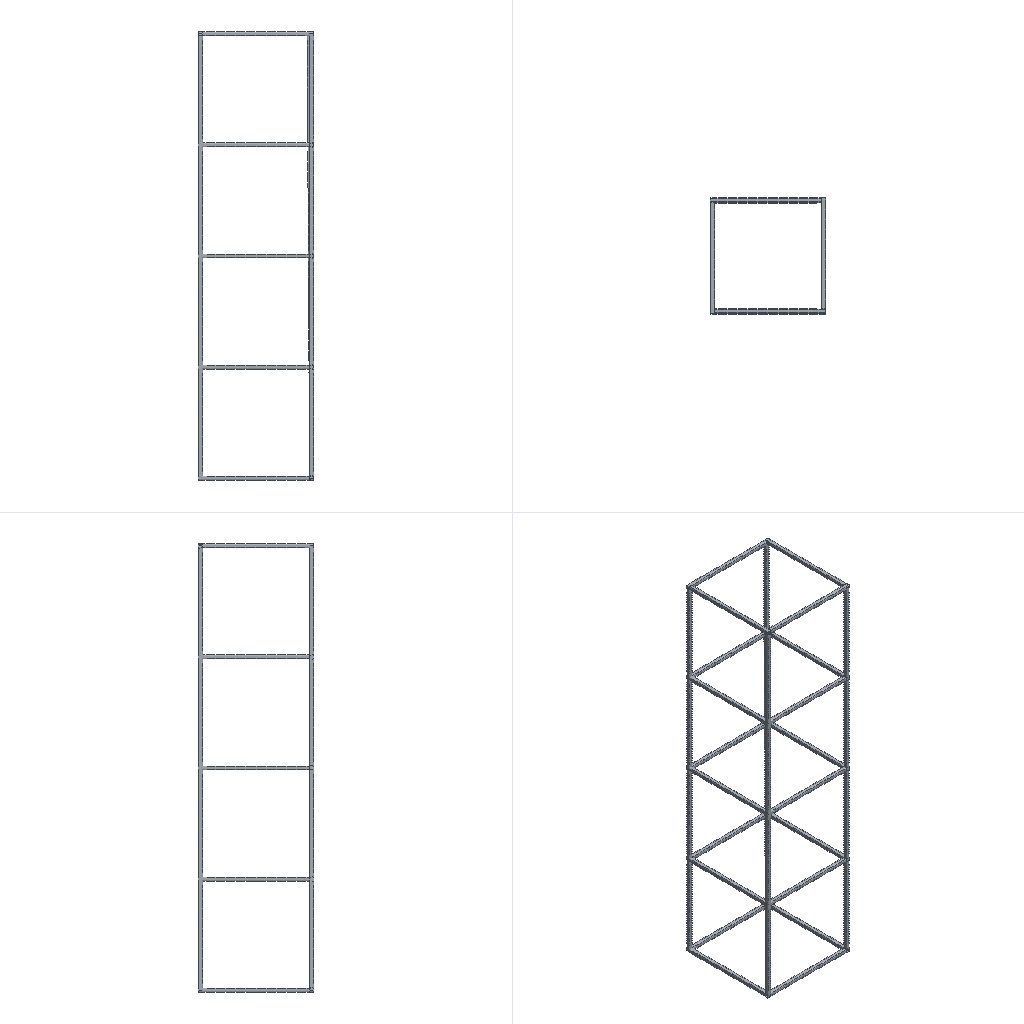Simulation study | ansys workbench
Ansys APDL input file, long lists of numbers shortened:
/batch
/config,noeldb,1     ! force off writing results to database
*get,_wallstrt,active,,time,wall
! ANSYS input file written by Workbench version 2022 R1
! File used for geometry attach:
/title,wbnew--____ (A5)
! ****** Begin Custom Load Command Snippet ******
/COM, ACT Extensions:
/COM,     LSDYNA, 2021.1
/COM,
! ****** End   Custom Load Command Snippet ******
*DIM,_wb_ProjectScratch_dir,string,248
_wb_ProjectScratch_dir(1) = ''
*DIM,_wb_SolverFiles_dir,string,248
_wb_SolverFiles_dir(1) = ''
*DIM,_wb_userfiles_dir,string,248
_wb_userfiles_dir(1) = ''
/com,--- Data in consistent NMM units. See Solving Units in the help system for more information.
/units,MPA
/nopr
/wb,file,start              !  signify a WB generated input file
/prep7
! Turn off shape checking because checks already performed inside WB mesher.
! See help system for more information.
SHPP,OFF,,NOWARN
/nolist
etcon,set             ! allow ANSYS to choose best KEYOP's for 180x elements, resets any applicable keyopt to MAPDL defaults
/com,*********** Nodes for the whole assembly ***********
nblock,3,,335992
(1i9,3e20.9e3)
        1     2.400000000E+02     2.588284271E+02     8.828427125E+00
! (305447 more lines like these left out)
-1
/wb,elem,start            !  set before creation of elements
/com,*********** Elements for Body 1 "__-FreeParts|__ 20 X 20 X 2.0(1)[4]" ***********
et,1,186
keyo,1,2,1          ! set full integration on SOLID186
eblock,19,solid,,1200
(19i9)
        1        1        1        1        0        0        0        0       20        0     9601    68809    69006    69556    69609    68858    68861    69555    69610
! (2399 more lines like these left out)
-1
/com,*********** Elements for Body 2 "__-FreeParts|__ 20 X 20 X 2.0(1)[2]" ***********
et,2,186
keyo,2,2,1          ! set full integration on SOLID186
eblock,19,solid,,1200
(19i9)
        2        2        2        2        0        0        0        0       20        0    13201    94369    94566    95116    95169    94418    94421    95115    95170
! (2399 more lines like these left out)
-1
/com,*********** Elements for Body 3 "__-FreeParts|__(__)1[9]" ***********
et,3,186
keyo,3,2,1          ! set full integration on SOLID186
eblock,19,solid,,1200
(19i9)
        3        3        3        3        0        0        0        0       20        0     6001    43099    44893    44700    43298    43246    44896    44699    43297
! (2399 more lines like these left out)
-1
/com,*********** Elements for Body 4 "__-FreeParts|__ 20 X 20 X 2.0(2)[4]" ***********
et,4,186
keyo,4,2,1          ! set full integration on SOLID186
eblock,19,solid,,1200
(19i9)
        4        4        4        4        0        0        0        0       20        0     3601    26359    27411    27360    26558    26506    27556    27359    26557
! (2399 more lines like these left out)
-1
/com,*********** Elements for Body 5 "__-FreeParts|__ 20 X 20 X 2.0(2)[2]" ***********
et,5,186
keyo,5,2,1          ! set full integration on SOLID186
eblock,19,solid,,1200
(19i9)
        5        5        5        5        0        0        0        0       20        0    15601   110860   112159   112156   111106   110958   112160   112153   111105
! (2399 more lines like these left out)
-1
! (19 more sections like these left out)
/wb,elem,end               !  done creating elements
/com,*********** Send User Defined Coordinate System(s) ***********
csys,0
toffst,273.15,  ! Temperature offset from absolute zero
/com,*********** Set Reference Temperature ***********
tref,22.
/wb,mat,start              !  starting to send materials
/com,*********** Send Materials ***********
Temperature = 'TEMP' ! Temperature
MP,DENS,1,7.85e-09,	! tonne mm^-3
MP,ALPX,1,1.2e-05,	! C^-1
MP,C,1,434000000,	! mm^2 s^-2 C^-1
MP,KXX,1,60.5,	! tonne mm s^-3 C^-1
MP,RSVX,1,0.00017,	! ohm mm
MP,EX,1,200000,	! tonne s^-2 mm^-1
MP,NUXY,1,0.3,
MP,MURX,1,10000,
Temperature = 'TEMP' ! Temperature
MP,DENS,2,7.85e-09,	! tonne mm^-3
MP,ALPX,2,1.2e-05,	! C^-1
MP,C,2,434000000,	! mm^2 s^-2 C^-1
MP,KXX,2,60.5,	! tonne mm s^-3 C^-1
MP,RSVX,2,0.00017,	! ohm mm
MP,EX,2,200000,	! tonne s^-2 mm^-1
MP,NUXY,2,0.3,
MP,MURX,2,10000,
Temperature = 'TEMP' ! Temperature
MP,DENS,3,7.85e-09,	! tonne mm^-3
MP,ALPX,3,1.2e-05,	! C^-1
MP,C,3,434000000,	! mm^2 s^-2 C^-1
MP,KXX,3,60.5,	! tonne mm s^-3 C^-1
MP,RSVX,3,0.00017,	! ohm mm
MP,EX,3,200000,	! tonne s^-2 mm^-1
MP,NUXY,3,0.3,
MP,MURX,3,10000,
Temperature = 'TEMP' ! Temperature
MP,DENS,4,7.85e-09,	! tonne mm^-3
MP,ALPX,4,1.2e-05,	! C^-1
MP,C,4,434000000,	! mm^2 s^-2 C^-1
MP,KXX,4,60.5,	! tonne mm s^-3 C^-1
MP,RSVX,4,0.00017,	! ohm mm
MP,EX,4,200000,	! tonne s^-2 mm^-1
MP,NUXY,4,0.3,
MP,MURX,4,10000,
Temperature = 'TEMP' ! Temperature
MP,DENS,5,7.85e-09,	! tonne mm^-3
MP,ALPX,5,1.2e-05,	! C^-1
MP,C,5,434000000,	! mm^2 s^-2 C^-1
MP,KXX,5,60.5,	! tonne mm s^-3 C^-1
MP,RSVX,5,0.00017,	! ohm mm
MP,EX,5,200000,	! tonne s^-2 mm^-1
MP,NUXY,5,0.3,
MP,MURX,5,10000,
Temperature = 'TEMP' ! Temperature
MP,DENS,6,7.85e-09,	! tonne mm^-3
MP,ALPX,6,1.2e-05,	! C^-1
MP,C,6,434000000,	! mm^2 s^-2 C^-1
MP,KXX,6,60.5,	! tonne mm s^-3 C^-1
MP,RSVX,6,0.00017,	! ohm mm
MP,EX,6,200000,	! tonne s^-2 mm^-1
MP,NUXY,6,0.3,
MP,MURX,6,10000,
Temperature = 'TEMP' ! Temperature
MP,DENS,7,7.85e-09,	! tonne mm^-3
MP,ALPX,7,1.2e-05,	! C^-1
MP,C,7,434000000,	! mm^2 s^-2 C^-1
MP,KXX,7,60.5,	! tonne mm s^-3 C^-1
MP,RSVX,7,0.00017,	! ohm mm
MP,EX,7,200000,	! tonne s^-2 mm^-1
MP,NUXY,7,0.3,
MP,MURX,7,10000,
Temperature = 'TEMP' ! Temperature
MP,DENS,8,7.85e-09,	! tonne mm^-3
MP,ALPX,8,1.2e-05,	! C^-1
MP,C,8,434000000,	! mm^2 s^-2 C^-1
MP,KXX,8,60.5,	! tonne mm s^-3 C^-1
MP,RSVX,8,0.00017,	! ohm mm
MP,EX,8,200000,	! tonne s^-2 mm^-1
MP,NUXY,8,0.3,
MP,MURX,8,10000,
Temperature = 'TEMP' ! Temperature
MP,DENS,9,7.85e-09,	! tonne mm^-3
MP,ALPX,9,1.2e-05,	! C^-1
MP,C,9,434000000,	! mm^2 s^-2 C^-1
MP,KXX,9,60.5,	! tonne mm s^-3 C^-1
MP,RSVX,9,0.00017,	! ohm mm
MP,EX,9,200000,	! tonne s^-2 mm^-1
! (137 more lines like these left out)
/wb,mat,end                !  done sending materials
!************************* Model Summary ********************
!__-FreeParts|__ 20 X 20 X 2.0(1)[4],	结构钢,	matid,	1
!__-FreeParts|__ 20 X 20 X 2.0(1)[2],	结构钢,	matid,	2
!__-FreeParts|__(__)1[9],	结构钢,	matid,	3
!__-FreeParts|__ 20 X 20 X 2.0(2)[4],	结构钢,	matid,	4
!__-FreeParts|__ 20 X 20 X 2.0(2)[2],	结构钢,	matid,	5
!__-FreeParts|__(__)1[3],	结构钢,	matid,	6
!__-FreeParts|__(__)1[8],	结构钢,	matid,	7
!__-FreeParts|__ 20 X 20 X 2.0(1)[3],	结构钢,	matid,	8
!__-FreeParts|__(__)1[12],	结构钢,	matid,	9
!__-FreeParts|__(__)1[2],	结构钢,	matid,	10
!__-FreeParts|__(__)1[4],	结构钢,	matid,	11
!__-FreeParts|__ 20 X 20 X 2.0(3)[3],	结构钢,	matid,	12
!__-FreeParts|__ 20 X 20 X 2.0(2)[3],	结构钢,	matid,	13
!__-FreeParts|__ 20 X 20 X 2.0(1)[1],	结构钢,	matid,	14
!__-FreeParts|__(__)1[10],	结构钢,	matid,	15
!__-FreeParts|__(__)1[6],	结构钢,	matid,	16
!__-FreeParts|__ 20 X 20 X 2.0(3)[4],	结构钢,	matid,	17
!__-FreeParts|__ 20 X 20 X 2.0(3)[1],	结构钢,	matid,	18
!__-FreeParts|__ 20 X 20 X 2.0(2)[1],	结构钢,	matid,	19
!__-FreeParts|__(__)1[5],	结构钢,	matid,	20
!__-FreeParts|__(__)1[1],	结构钢,	matid,	21
!__-FreeParts|__ 20 X 20 X 2.0(3)[2],	结构钢,	matid,	22
!__-FreeParts|__(__)1[11],	结构钢,	matid,	23
!__-FreeParts|__(__)1[7],	结构钢,	matid,	24
!************************* End Model Summary ********************
! get the diagonal of the bounding box. Needed later for other things
*get,_xmin,node,,mnloc,x
*get,_ymin,node,,mnloc,y
*get,_zmin,node,,mnloc,z
*get,_xmax,node,,mxloc,x
*get,_ymax,node,,mxloc,y
*get,_zmax,node,,mxloc,z
_ASMDIAG=(_xmax-_xmin)*(_xmax-_xmin)+(_ymax-_ymin)*(_ymax-_ymin)+(_zmax-_zmin)*(_zmax-_zmin)
_ASMDIAG=SQRT(_ASMDIAG)
/wb,contact,start          !  starting to send contact
/com,*********** Create Contact "接触区域" ***********
/com,            Real Constant Set For Above Contact Is 26 & 25
*set,tid,26
*set,cid,25
r,tid
r,cid
et,tid,170
et,cid,174
eblock,10,,,32
(15i9)
   130825       26       26       26        0    69958    69959    68173    68174    75443    70648    70646    70651
! (31 more lines like these left out)
-1
eblock,10,,,32
(15i9)
   130857       25       25       25        0    69958    69959    68173    68174    75443    70648    70646    70651
! (31 more lines like these left out)
-1
eblock,10,,,24
(15i9)
   130889       25       26       25        0    86596    86046    85849    86649    90198    89608    89609    91689
! (23 more lines like these left out)
-1
eblock,10,,,24
(15i9)
   130913       26       25       26        0    86596    86046    85849    86649    90198    89608    89609    91689
! (23 more lines like these left out)
-1
keyo,cid,8,2               ! auto create asymmetric contact (from Program Controlled setting)
keyo,cid,10,0              ! adjust contact stiffness each NR iteration (from Program Controlled setting)
keyo,cid,12,5              ! bonded always
keyo,cid,18,1              ! small sliding turned on by application
keyo,cid,2,0               ! augmented Lagrange (from Program Controlled setting)
keyo,cid,4,0               ! on Gauss point (from Program Controlled setting)
keyo,cid,9,1               ! ignore initial gaps/penetration
keyo,cid,7,0               ! No Prediction
rmod,tid,3,10.      ! FKN
rmod,tid,5,0.       ! ICONT
rmod,tid,6,0.       ! PINB
rmod,tid,10,0.      ! CNOF
rmod,tid,12,0.      ! FKT
rmod,tid,36,95      ! WB DSID
rmod,cid,3,10.      ! FKN
rmod,cid,5,0.       ! ICONT
rmod,cid,6,0.       ! PINB
rmod,cid,10,0.      ! CNOF
rmod,cid,12,0.      ! FKT
rmod,cid,36,95      ! WB DSID
/com,*********** Create Contact "接触区域 2" ***********
/com,            Real Constant Set For Above Contact Is 28 & 27
*set,tid,28
*set,cid,27
r,tid
r,cid
et,tid,170
et,cid,174
eblock,10,,,120
(15i9)
   130937       28       28       28        0    68456    68347    68344    68455    71194    71183    71184    71513
! (119 more lines like these left out)
-1
eblock,10,,,120
(15i9)
   131057       27       27       27        0    68456    68347    68344    68455    71194    71183    71184    71513
! (119 more lines like these left out)
-1
eblock,10,,,108
(15i9)
   131177       27       28       27        0   145290   144889   144888   144887   154611   154608   154606   154607
! (107 more lines like these left out)
-1
eblock,10,,,108
(15i9)
   131285       28       27       28        0   145290   144889   144888   144887   154611   154608   154606   154607
! (107 more lines like these left out)
-1
keyo,cid,8,2               ! auto create asymmetric contact (from Program Controlled setting)
keyo,cid,10,0              ! adjust contact stiffness each NR iteration (from Program Controlled setting)
keyo,cid,12,5              ! bonded always
keyo,cid,18,1              ! small sliding turned on by application
keyo,cid,2,0               ! augmented Lagrange (from Program Controlled setting)
keyo,cid,4,0               ! on Gauss point (from Program Controlled setting)
keyo,cid,9,1               ! ignore initial gaps/penetration
keyo,cid,7,0               ! No Prediction
rmod,tid,3,10.      ! FKN
rmod,tid,5,0.       ! ICONT
rmod,tid,6,0.       ! PINB
rmod,tid,10,0.      ! CNOF
rmod,tid,12,0.      ! FKT
rmod,tid,36,98      ! WB DSID
rmod,cid,3,10.      ! FKN
rmod,cid,5,0.       ! ICONT
rmod,cid,6,0.       ! PINB
rmod,cid,10,0.      ! CNOF
rmod,cid,12,0.      ! FKT
rmod,cid,36,98      ! WB DSID
/com,*********** Create Contact "接触区域 3" ***********
/com,            Real Constant Set For Above Contact Is 30 & 29
*set,tid,30
*set,cid,29
r,tid
r,cid
et,tid,170
et,cid,174
eblock,10,,,24
(15i9)
   131393       30       30       30        0    69556    69006    68809    69609    73158    72568    72569    74649
! (23 more lines like these left out)
-1
eblock,10,,,24
(15i9)
   131417       29       29       29        0    69556    69006    68809    69609    73158    72568    72569    74649
! (23 more lines like these left out)
-1
eblock,10,,,32
(15i9)
   131441       29       30       29        0     1852     1845     1844     1853     7377     7374     7375     7389
! (31 more lines like these left out)
-1
eblock,10,,,32
(15i9)
   131473       30       29       30        0     1852     1845     1844     1853     7377     7374     7375     7389
! (31 more lines like these left out)
-1
keyo,cid,8,2               ! auto create asymmetric contact (from Program Controlled setting)
keyo,cid,10,0              ! adjust contact stiffness each NR iteration (from Program Controlled setting)
keyo,cid,12,5              ! bonded always
keyo,cid,18,1              ! small sliding turned on by application
keyo,cid,2,0               ! augmented Lagrange (from Program Controlled setting)
keyo,cid,4,0               ! on Gauss point (from Program Controlled setting)
keyo,cid,9,1               ! ignore initial gaps/penetration
keyo,cid,7,0               ! No Prediction
rmod,tid,3,10.      ! FKN
rmod,tid,5,0.       ! ICONT
rmod,tid,6,0.       ! PINB
rmod,tid,10,0.      ! CNOF
rmod,tid,12,0.      ! FKT
rmod,tid,36,101     ! WB DSID
rmod,cid,3,10.      ! FKN
rmod,cid,5,0.       ! ICONT
rmod,cid,6,0.       ! PINB
rmod,cid,10,0.      ! CNOF
rmod,cid,12,0.      ! FKT
rmod,cid,36,101     ! WB DSID
/com,*********** Create Contact "接触区域 4" ***********
/com,            Real Constant Set For Above Contact Is 32 & 31
*set,tid,32
*set,cid,31
r,tid
r,cid
et,tid,170
et,cid,174
eblock,10,,,24
(15i9)
   131505       32       32       32        0    69556    69006    68809    69609    73158    72568    72569    74649
! (23 more lines like these left out)
-1
eblock,10,,,24
(15i9)
   131529       31       31       31        0    69556    69006    68809    69609    73158    72568    72569    74649
! (23 more lines like these left out)
-1
eblock,10,,,24
(15i9)
   131553       31       32       31        0   207167   206966   206965   207166   222469   222465   222466   223066
! (23 more lines like these left out)
-1
eblock,10,,,24
(15i9)
   131577       32       31       32        0   207167   206966   206965   207166   222469   222465   222466   223066
! (23 more lines like these left out)
-1
keyo,cid,8,2               ! auto create asymmetric contact (from Program Controlled setting)
keyo,cid,10,0              ! adjust contact stiffness each NR iteration (from Program Controlled setting)
keyo,cid,12,5              ! bonded always
keyo,cid,18,1              ! small sliding turned on by application
keyo,cid,2,0               ! augmented Lagrange (from Program Controlled setting)
keyo,cid,4,0               ! on Gauss point (from Program Controlled setting)
keyo,cid,9,1               ! ignore initial gaps/penetration
keyo,cid,7,0               ! No Prediction
rmod,tid,3,10.      ! FKN
rmod,tid,5,0.       ! ICONT
rmod,tid,6,0.       ! PINB
rmod,tid,10,0.      ! CNOF
rmod,tid,12,0.      ! FKT
rmod,tid,36,104     ! WB DSID
rmod,cid,3,10.      ! FKN
rmod,cid,5,0.       ! ICONT
rmod,cid,6,0.       ! PINB
rmod,cid,10,0.      ! CNOF
rmod,cid,12,0.      ! FKT
rmod,cid,36,104     ! WB DSID
/com,*********** Create Contact "接触区域 5" ***********
/com,            Real Constant Set For Above Contact Is 34 & 33
*set,tid,34
*set,cid,33
r,tid
r,cid
et,tid,170
et,cid,174
eblock,10,,,24
(15i9)
   131601       34       34       34        0    95116    94566    94369    95169    98718    98128    98129   100209
! (23 more lines like these left out)
-1
eblock,10,,,24
(15i9)
   131625       33       33       33        0    95116    94566    94369    95169    98718    98128    98129   100209
! (23 more lines like these left out)
-1
eblock,10,,,32
(15i9)
   131649       33       34       33        0    87052    87045    87044    87053    92578    92575    92576    92589
! (31 more lines like these left out)
-1
eblock,10,,,32
(15i9)
   131681       34       33       34        0    87052    87045    87044    87053    92578    92575    92576    92589
! (31 more lines like these left out)
-1
keyo,cid,8,2               ! auto create asymmetric contact (from Program Controlled setting)
keyo,cid,10,0              ! adjust contact stiffness each NR iteration (from Program Controlled setting)
keyo,cid,12,5              ! bonded always
keyo,cid,18,1              ! small sliding turned on by application
keyo,cid,2,0               ! augmented Lagrange (from Program Controlled setting)
keyo,cid,4,0               ! on Gauss point (from Program Controlled setting)
keyo,cid,9,1               ! ignore initial gaps/penetration
keyo,cid,7,0               ! No Prediction
rmod,tid,3,10.      ! FKN
rmod,tid,5,0.       ! ICONT
rmod,tid,6,0.       ! PINB
rmod,tid,10,0.      ! CNOF
rmod,tid,12,0.      ! FKT
rmod,tid,36,107     ! WB DSID
rmod,cid,3,10.      ! FKN
rmod,cid,5,0.       ! ICONT
rmod,cid,6,0.       ! PINB
rmod,cid,10,0.      ! CNOF
rmod,cid,12,0.      ! FKT
rmod,cid,36,107     ! WB DSID
! (55 more sections like these left out)
/wb,contact,end            !  done creating contacts
/golist
/wb,load,start             !  starting to send loads
/com,*********** Fixed Supports ***********
CMBLOCK,_FIXEDSU,NODE,     2836
(8i10)
         2         3         4         5         6      2149      2150      2151
! (354 more lines like these left out)
cmsel,s,_FIXEDSU
d,all,all
nsel,all
/com,*********** Define Force Using Surface Effect Elements ***********
local,12,0,0.,0.,0.,0.,0.,0.
csys,0
et,145,154
eblock,10,,,2604
(15i9)
   147347      145      145      145       12   273015   272212   271603   271602   283386   281367   281364   281365
! (2603 more lines like these left out)
-1
esel,s,type,,145
keyop,145,2,1                ! Apply load in local coordinate system
keyop,145,7,1                ! Use original area so load is constant in large deformation
esel,all
/gst,on,on
fini
*get,_numnode,node,0,count
*get,_numelem,elem,0,count
*get, _MAXELEMNUM, elem, 0, NUM, MAX
*get, _MAXNODENUM, node, 0, NUM, MAX
*get, _MAXELEMTYPE, etyp, 0, NUM, MAX
*get, _MAXREALCONST, real, 0, NUM, MAX
/go
/wb,load,end               !  done creating loads
/com,--- Number of total nodes = %_numnode%
/com,--- Number of contact elements = 19126
/com,--- Number of spring elements = 0
/com,--- Number of bearing elements = 0
/com,--- Number of solid elements = 43224
/com,--- Number of condensed parts = 0
/com,--- Number of total elements = %_numelem%
*get,_wallbsol,active,,time,wall
/com,****************************************************************************
/com,*************************    SOLUTION       ********************************
/com,****************************************************************************
/solu
antype,0                   ! static analysis
_thickRatio=  0     ! Ratio of thick parts in the model
eqsl,sparse,,,,,1
cntr,print,1               ! print out contact info and also make no initial contact an error
dmpoption,emat,no             ! Don't combine emat file for DANSYS
dmpoption,esav,no             ! Don't combine esav file for DANSYS
nldiag,cont,iter           ! print out contact info each equilibrium iteration
rescontrol,,none                 ! Do not keep any restart files
/com,****************************************************
/com,******************* SOLVE FOR LS 1 OF 1 ****************
esel,s,type,,145
nsle
sfe,all,1,pres,1,0.
sfe,all,2,pres,1,-6.41022770017667e-002
sfe,all,3,pres,1,0.
nsel,all
esel,all
/nopr
/gopr
nsub,1,1,1
time,1.
outres,erase
outres,all,none
outres,nsol,all,
outres,rsol,all
outres,eangl,all
outres,etmp,all
outres,veng,all
outres,strs,all,
outres,epel,all,
outres,eppl,all,
outres,cont,all,
! *********** WB SOLVE COMMAND ***********
! check interactive state
*get,ANSINTER_,active,,int
*if,ANSINTER_,ne,0,then
/eof
*endif
solve
/com *************** Write FE CONNECTORS *********
CEWRITE,file,ce,,INTE
/com,****************************************************
/com,*************** FINISHED SOLVE FOR LS 1 *************
*get,_wallasol,active,,time,wall
/nopr
*get,_numnode,node,0,count
*get,_numelem,elem,0,count
*get, _MAXELEMNUM, elem, 0, NUM, MAX
*get, _MAXNODENUM, node, 0, NUM, MAX,,,INTERNAL
*get, _MAXELEMTYPE, etyp, 0, NUM, MAX
*get, _MAXREALCONST, real, 0, NUM, MAX
/gopr
/post1
xmlo,ENCODING,ISO-8859-1
xmlo,parm
/xml,parm,xml
fini
/gopr
*get,_walldone,active,,time,wall
_preptime=(_wallbsol-_wallstrt)*3600
_solvtime=(_wallasol-_wallbsol)*3600
_posttime=(_walldone-_wallasol)*3600
_totaltim=(_walldone-_wallstrt)*3600
*get,_dlbratio,active,0,solu,dlbr
*get,_combtime,active,0,solu,comb
*get,_ssmode,active,0,solu,ssmm
*get,_ndofs,active,0,solu,ndof
*get,_sol_end_time,active,0,set,time
*if,_sol_end_time,eq,1.,then
/fclean				!clean distributed files
*endif
/com,--- Total number of nodes = %_numnode%
/com,--- Total number of elements = %_numelem%
/com,--- Element load balance ratio = %_dlbratio%
/com,--- Time to combine distributed files = %_combtime%
/com,--- Sparse memory mode = %_ssmode%
/com,--- Number of DOF = %_ndofs%
/wb,file,end               ! done with WB generated input